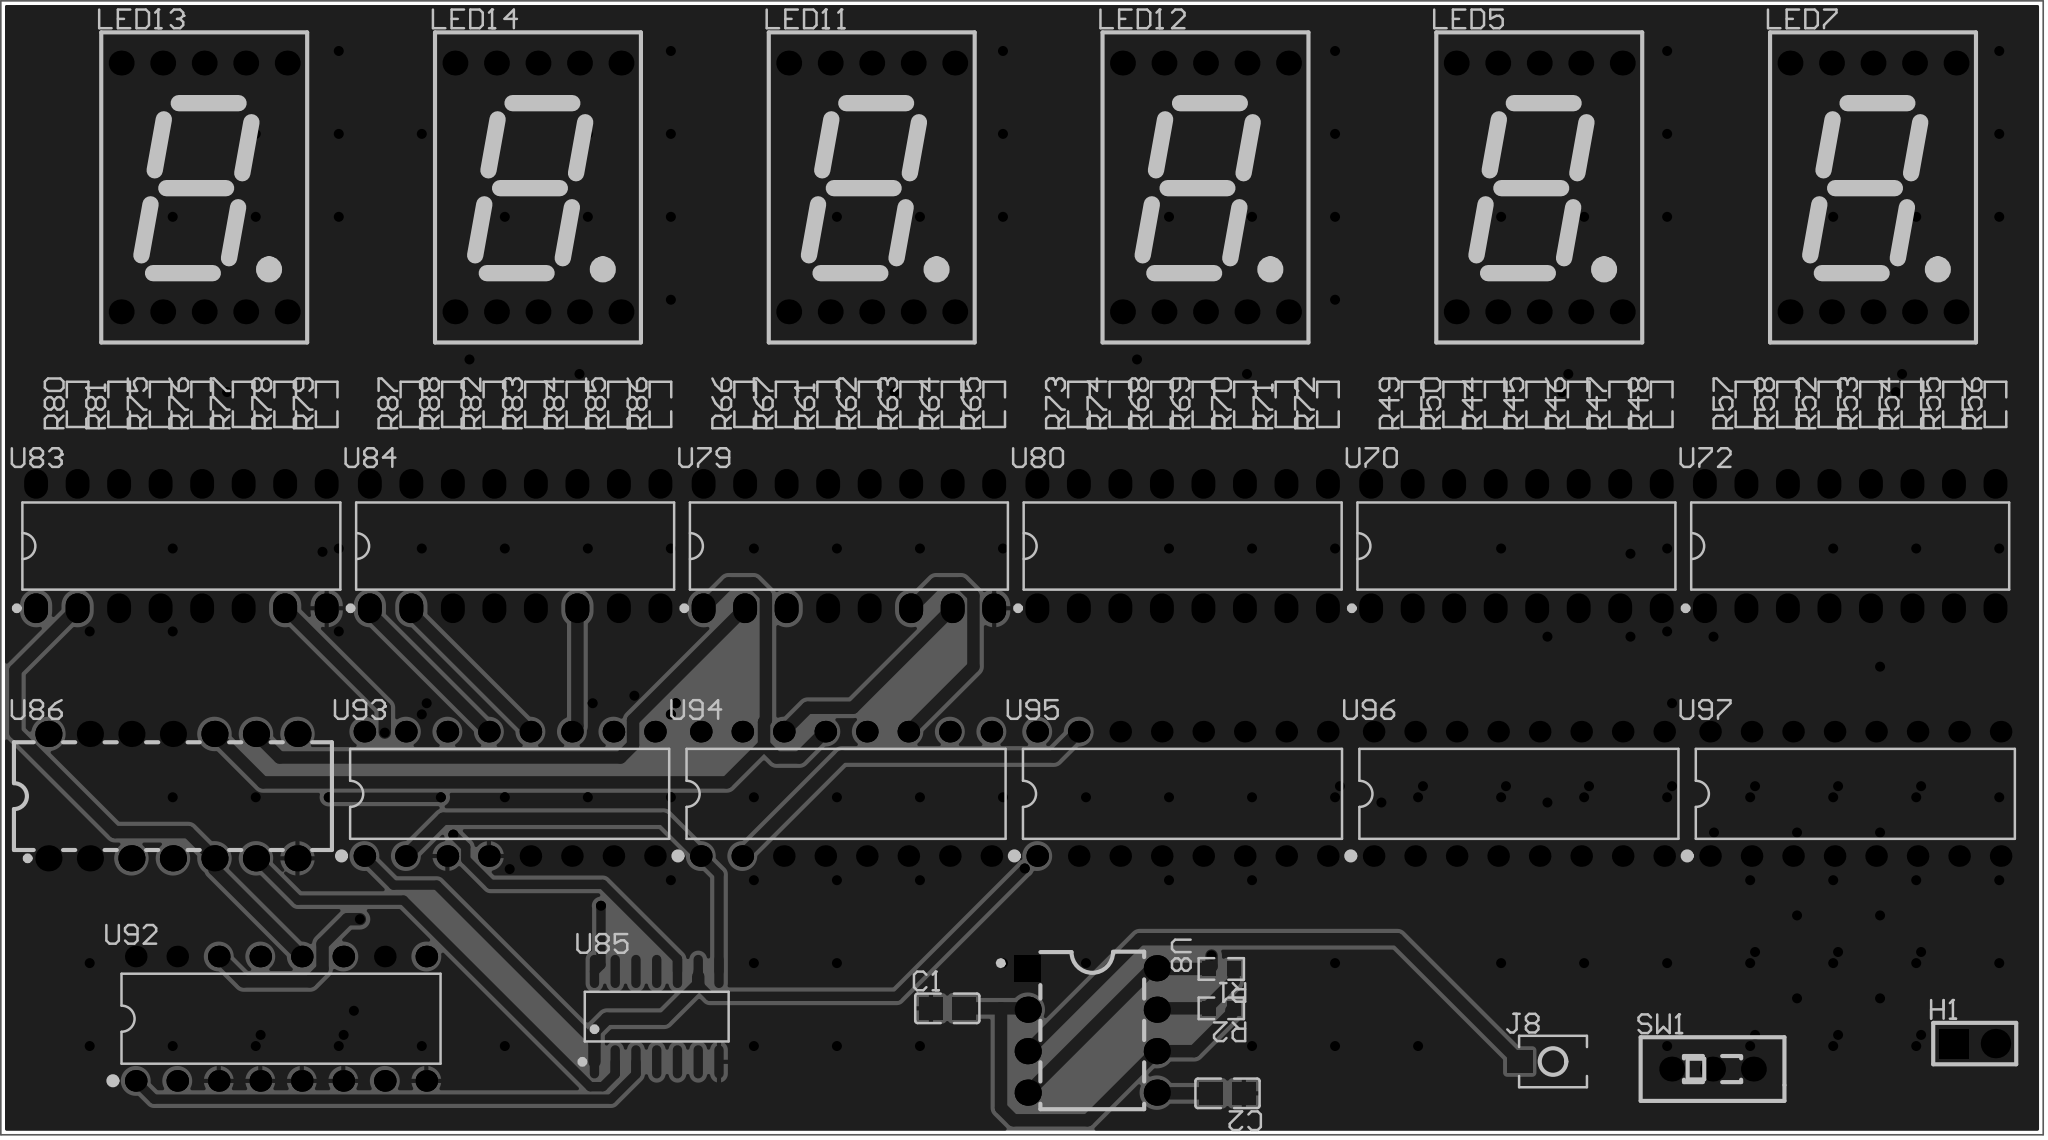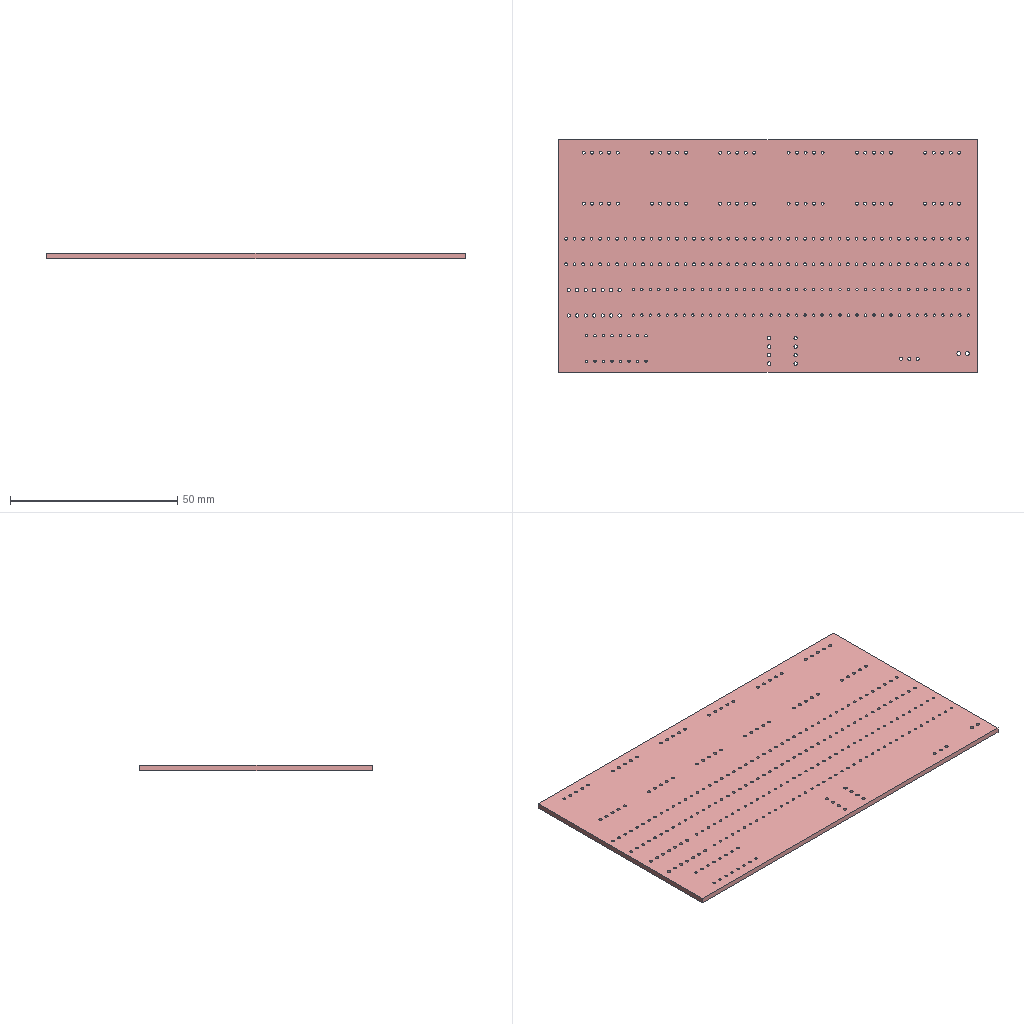Circuit board layout | Altium Designer | box 125 x 69.5 x 1.6 mm
Layer stack:
# Altium Designer layer stack of  (unit mm; dielectric type: 0 none, 1 core, 2 prepreg, 3 surface material)
index,name,kind,layer,copper_thickness_mm,dielectric_type,dielectric_thickness_mm,dielectric_material,dielectric_constant
0,Top Paste Mask Layer,other,,,,,,
1,Top Silkscreen Layer,other,,,,,,
2,Top Solder Mask Layer,dielectric,,,3,0.01,,3.3
3,Top Layer,copper,Top Layer,0.035,,,,
4,Dielectric1,dielectric,,,3,1.51,FR4,4.5
5,Bottom Layer,copper,Bottom Layer,0.035,,,,
6,Bottom Solder Mask Layer,dielectric,,,3,0.01,,3.3
7,Bottom Silkscreen Layer,other,,,,,,
8,Bottom Paste Mask Layer,other,,,,,,
# drill layer pairs: low layer,high layer
drill_pair,Top Layer,Bottom Layer
Part placement:
Designator,Comment,Layer,Footprint,Center-X(mm),Center-Y(mm),Rotation
C1,1uF,TopLayer,C0805,145.923,89.281,0
C2,10nF,TopLayer,C0805,163.068,84.074,180
H1,,TopLayer,HDR-TH_2P-P2.54-V-M-1,208.788,87.122,0
J8,轻触按键3*4*H,TopLayer,SW-SMD_L4.0-W2.9-LS5.0,182.986,86.022,0
LED5,,TopLayer,LED-SEG-TH_10P-L12.6-W19.0-P2.54-S15.24-BL,182.143,139.573,0
LED7,,TopLayer,LED-SEG-TH_10P-L12.6-W19.0-P2.54-S15.24-BL,202.565,139.573,0
LED11,,TopLayer,LED-SEG-TH_10P-L12.6-W19.0-P2.54-S15.24-BL,141.299,139.573,0
LED12,,TopLayer,LED-SEG-TH_10P-L12.6-W19.0-P2.54-S15.24-BL,161.721,139.573,0
LED13,,TopLayer,LED-SEG-TH_10P-L12.6-W19.0-P2.54-S15.24-BL,100.456,139.573,0
LED14,,TopLayer,LED-SEG-TH_10P-L12.6-W19.0-P2.54-S15.24-BL,120.877,139.573,0
R1,10k,TopLayer,R0603,162.687,91.694,180
R2,2.2k,TopLayer,R0603,162.687,89.281,180
R44,250,TopLayer,R0603,179.477,126.282,90
R45,250,TopLayer,R0603,182.017,126.282,90
R46,250,TopLayer,R0603,184.557,126.282,90
R47,250,TopLayer,R0603,187.096,126.282,90
R48,250,TopLayer,R0603,189.636,126.282,90
R49,250,TopLayer,R0603,174.398,126.282,90
R50,250,TopLayer,R0603,176.938,126.282,90
R52,250,TopLayer,R0603,199.899,126.282,90
R53,250,TopLayer,R0603,202.439,126.282,90
R54,250,TopLayer,R0603,204.979,126.282,90
R55,250,TopLayer,R0603,207.518,126.282,90
R56,250,TopLayer,R0603,210.058,126.282,90
R57,250,TopLayer,R0603,194.82,126.282,90
R58,250,TopLayer,R0603,197.36,126.282,90
R61,250,TopLayer,R0603,138.634,126.282,90
R62,250,TopLayer,R0603,141.173,126.282,90
R63,250,TopLayer,R0603,143.713,126.282,90
R64,250,TopLayer,R0603,146.253,126.282,90
R65,250,TopLayer,R0603,148.792,126.282,90
R66,250,TopLayer,R0603,133.554,126.282,90
R67,250,TopLayer,R0603,136.094,126.282,90
R68,250,TopLayer,R0603,159.056,126.282,90
R69,250,TopLayer,R0603,161.595,126.282,90
R70,250,TopLayer,R0603,164.135,126.282,90
R71,250,TopLayer,R0603,166.675,126.282,90
R72,250,TopLayer,R0603,169.214,126.282,90
R73,250,TopLayer,R0603,153.976,126.282,90
R74,250,TopLayer,R0603,156.516,126.282,90
R75,250,TopLayer,R0603,97.79,126.282,90
R76,250,TopLayer,R0603,100.33,126.282,90
R77,250,TopLayer,R0603,102.869,126.282,90
R78,250,TopLayer,R0603,105.409,126.282,90
R79,250,TopLayer,R0603,107.948,126.282,90
R80,250,TopLayer,R0603,92.711,126.282,90
R81,250,TopLayer,R0603,95.25,126.282,90
R82,250,TopLayer,R0603,118.212,126.282,90
R83,250,TopLayer,R0603,120.751,126.282,90
R84,250,TopLayer,R0603,123.291,126.282,90
R85,250,TopLayer,R0603,125.831,126.282,90
R86,250,TopLayer,R0603,128.37,126.282,90
R87,250,TopLayer,R0603,113.133,126.282,90
R88,250,TopLayer,R0603,115.672,126.282,90
SW1,开关,TopLayer,SW-TH_SS-12D01-GX,192.746,85.56,0
U8,NE555PE4,TopLayer,PDIP-8_L9.6-W6.4-P2.54-LS7.9-BL-1,154.794,87.927,270
U70,SN74LS48N,TopLayer,DIP-16_L19.3-W6.4-P2.54-LS7.6-BL,180.746,117.602,0
U72,SN74LS48N,TopLayer,DIP-16_L19.3-W6.4-P2.54-LS7.6-BL,201.168,117.602,0
U79,SN74LS48N,TopLayer,DIP-16_L19.3-W6.4-P2.54-LS7.6-BL,139.902,117.602,0
U80,SN74LS48N,TopLayer,DIP-16_L19.3-W6.4-P2.54-LS7.6-BL,160.324,117.602,0
U83,SN74LS48N,TopLayer,DIP-16_L19.3-W6.4-P2.54-LS7.6-BL,99.058,117.602,0
U84,SN74LS48N,TopLayer,DIP-16_L19.3-W6.4-P2.54-LS7.6-BL,119.48,117.602,0
U85,SN74LS08DR(LX),TopLayer,SOIC-14_L8.7-W3.9-P1.27-LS6.0-BL,128.143,88.773,0
U86,SN74LS00N(LX),TopLayer,PDIP-14_L19.3-W6.4-P2.54-LS7.9-BL,98.542,102.281,0
U92,SN74LS160N(LX),TopLayer,DIP-16_L19.4-W6.4-P2.54-S7.6-BL,105.156,88.646,0
U93,SN74LS160N(LX),TopLayer,DIP-16_L19.4-W6.4-P2.54-S7.6-BL,119.145,102.421,0
U94,SN74LS160N(LX),TopLayer,DIP-16_L19.4-W6.4-P2.54-S7.6-BL,139.729,102.421,0
U95,SN74LS160N(LX),TopLayer,DIP-16_L19.4-W6.4-P2.54-S7.6-BL,160.314,102.421,0
U96,SN74LS160N(LX),TopLayer,DIP-16_L19.4-W6.4-P2.54-S7.6-BL,180.898,102.421,0
U97,SN74LS160N(LX),TopLayer,DIP-16_L19.4-W6.4-P2.54-S7.6-BL,201.483,102.421,0
Pad and via stacks:
# Altium Designer via and pad stacks of  (unit mm). Each distinct definition once, with the count of objects using it.
# via: kind,start_layer,end_layer,hole_mm,diameter_mm,mode(0 simple;1 top-mid-bottom;2 full stack),diameter_per_layer,count,example_net
# pad: kind,layer,hole_mm,hole_type(0 round;1 square;2 slot),plating,top_size,top_shape(1 round;2 rect;3 octagon;9 rounded rect),mid_size,bottom_size,mode,footprint,size_per_layer,count,example
pad,Top Layer,0,0,plated,1.41x1.35,2,1.41x1.35,1.41x1.35,0,C0805,,4,C1.2
pad,Top Layer,0,0,plated,1.53x1.36,2,1.53x1.36,1.53x1.36,0,SW-SMD_L4.0-W2.9-LS5.0,,2,J8.1
pad,Top Layer,0,0,plated,0.8065x0.864,2,0.8065x0.864,0.8065x0.864,0,R0603,,88,R1.2
pad,Top Layer,0,0,plated,0.574x2.038,1,0.574x2.038,0.574x2.038,0,SOIC-14_L8.7-W3.9-P1.27-LS6.0-BL,,14,U85.1
pad,Multi-Layer,1.1,0,plated,1.8x1.8,1,1.8x1.8,1.8x1.8,0,HDR-TH_2P-P2.54-V-M-1,,1,H1.2
pad,Multi-Layer,1.1,0,plated,1.8x1.8,2,1.8x1.8,1.8x1.8,0,HDR-TH_2P-P2.54-V-M-1,,1,H1.1
pad,Multi-Layer,0.9144,0,plated,1.524x1.524,1,1.524x1.524,1.524x1.524,0,LED-SEG-TH_10P-L12.6-W19.0-P2.54-S15.24-BL,,60,LED5.1
pad,Multi-Layer,0.9144,0,plated,1.524x1.524,1,1.524x1.524,1.524x1.524,0,SW-TH_SS-12D01-GX,,3,SW1.1
pad,Multi-Layer,1,0,plated,1.6x1.6,1,1.6x1.6,1.6x1.6,0,PDIP-8_L9.6-W6.4-P2.54-LS7.9-BL-1,,7,U8.8
pad,Multi-Layer,1,0,plated,1.6x1.6,2,1.6x1.6,1.6x1.6,0,PDIP-8_L9.6-W6.4-P2.54-LS7.9-BL-1,,1,U8.1
pad,Multi-Layer,0.8,0,plated,1.46x1.825,1,1.46x1.825,1.46x1.825,0,DIP-16_L19.3-W6.4-P2.54-LS7.6-BL,,96,U70.9
pad,Multi-Layer,1,0,plated,1.6x1.6,1,1.6x1.6,1.6x1.6,0,PDIP-14_L19.3-W6.4-P2.54-LS7.9-BL,,14,U86.9
pad,Multi-Layer,0.7,0,plated,1.32x1.32,1,1.32x1.32,1.32x1.32,0,DIP-16_L19.4-W6.4-P2.54-S7.6-BL,,96,U92.1
via,Top Layer,Bottom Layer,0.3048,0.61,0,,179,$1N58826
Copper pours:
name,layer,net,type(0 solid;1 hatched;2 none)
Top Layer-GND,Top Layer,GND,0
Bottom Layer-GND,Bottom Layer,GND,0
Design rules, without the lines most boards share:
# Altium Designer design rules of  (exported by Altium Designer, unit mm)
# columns: name | kind | enabled | priority | scope1 | scope2 | descriptor | typed fields (field=value)
copperThickness1oz_2 | 2 | enabled | 2 | All | All | Width Constraint (Min=5mil) (Max=100mil) (Preferred=30mil) (All) |
viaSize | 11 | enabled | 1 | All | All | Routing Via (MinHoleWidth=11.811mil) (MaxHoleWidth=248.032mil) (PreferredHoleWidth=12.008mil) (MinWidth=19.685mil) (MaxWidth=393.701mil) (PreferedWidth=24.016mil) (All) | via_min_hole=0.3 via_max_hole=6.3 via_preferred_diameter=0.61 via_preferred_hole=0.305
solderMaskExpansion | 13 | enabled | 2 | All | All | Solder Mask Expansion (Expansion =2.008mil) (All) | expansion=0.051